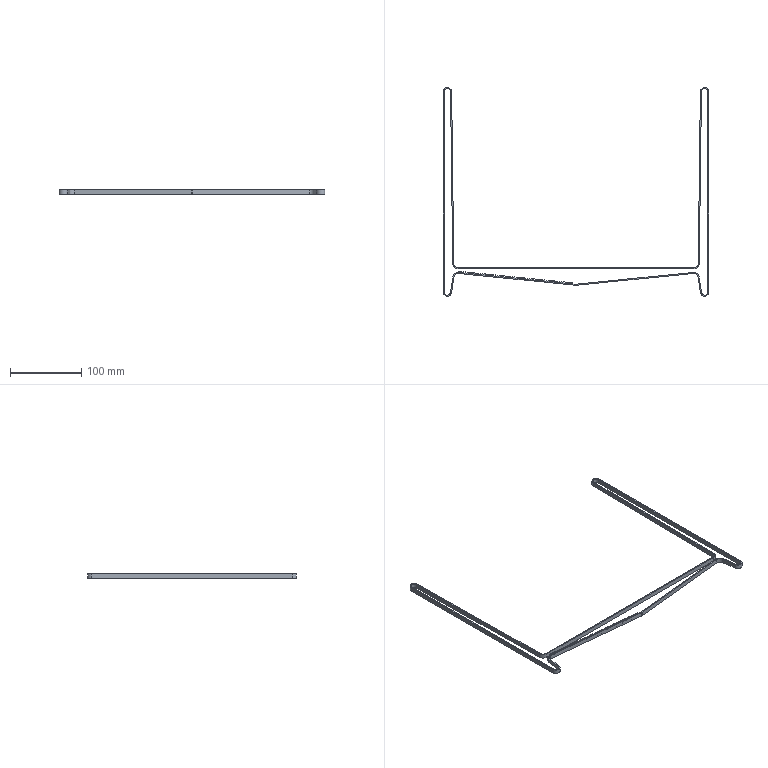Part | SolidWorks | features Extrusion 1, ICE 1, LPattern 1 | 1 solid | 254 faces | box 372 x 292 x 6 mm | volume 17336 mm3 | plane 236 | cylinder 18 | commonest cylinder face diameters 12 x9 15 x5 9 x4